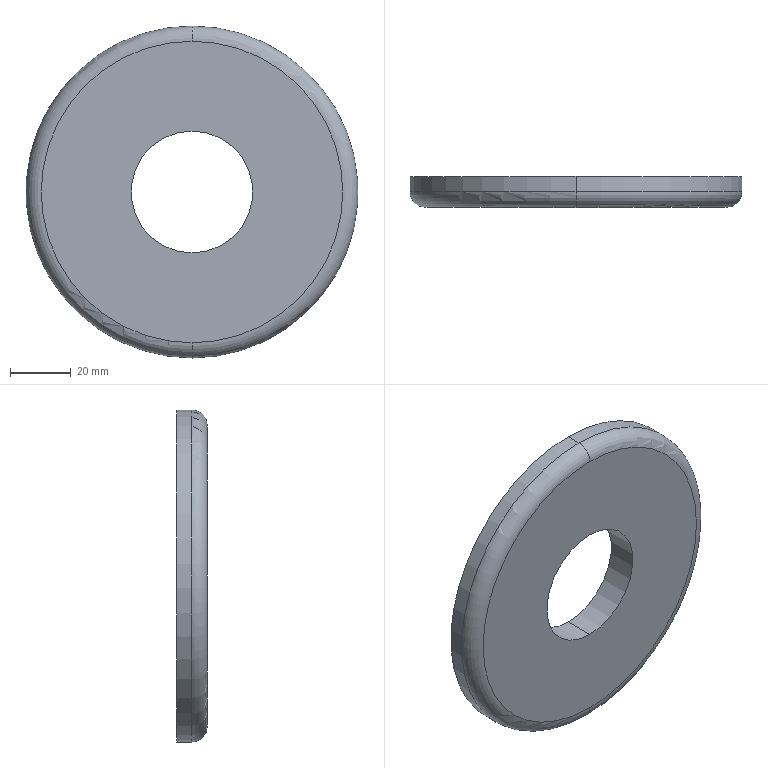Part | SolidWorks | features Revolution 1 | 1 solid | 8 faces | box 109 x 10 x 109 mm | volume 78947 mm3 | cylinder 4 | torus 2 | plane 2 | commonest cylinder face diameters 40 x2 109 x2
STEP:
#1=CARTESIAN_POINT('',(0.,-7.047,-20.));
#2=VERTEX_POINT('',#1);
#3=CARTESIAN_POINT('',(0.,-7.047,20.));
#4=VERTEX_POINT('',#3);
#5=CARTESIAN_POINT('',(0.,-7.047,0.));
#6=DIRECTION('',(0.,1.,0.));
#7=DIRECTION('',(0.,0.,1.));
#8=AXIS2_PLACEMENT_3D('',#5,#6,#7);
#9=CIRCLE('',#8,20.);
#10=EDGE_CURVE('',#2,#4,#9,.T.);
#11=ORIENTED_EDGE('',*,*,#10,.F.);
#12=CARTESIAN_POINT('',(0.,2.953,-20.));
#13=VERTEX_POINT('',#12);
#14=CARTESIAN_POINT('',(0.,51.821,-20.));
#15=DIRECTION('',(0.,1.,0.));
#16=VECTOR('',#15,1000.);
#17=LINE('',#14,#16);
#18=EDGE_CURVE('',#2,#13,#17,.T.);
#19=ORIENTED_EDGE('',*,*,#18,.T.);
#20=CARTESIAN_POINT('',(0.,2.953,20.));
#21=VERTEX_POINT('',#20);
#22=CARTESIAN_POINT('',(0.,2.953,0.));
#23=DIRECTION('',(0.,1.,0.));
#24=DIRECTION('',(0.,0.,1.));
#25=AXIS2_PLACEMENT_3D('',#22,#23,#24);
#26=CIRCLE('',#25,20.);
#27=EDGE_CURVE('',#13,#21,#26,.T.);
#28=ORIENTED_EDGE('',*,*,#27,.T.);
#29=CARTESIAN_POINT('',(0.,51.821,20.));
#30=DIRECTION('',(0.,1.,0.));
#31=VECTOR('',#30,1000.);
#32=LINE('',#29,#31);
#33=EDGE_CURVE('',#4,#21,#32,.T.);
#34=ORIENTED_EDGE('',*,*,#33,.F.);
#35=EDGE_LOOP('',(#11,#19,#28,#34));
#36=FACE_OUTER_BOUND('',#35,.T.);
#37=CARTESIAN_POINT('',(0.,51.821,0.));
#38=DIRECTION('',(0.,1.,0.));
#39=DIRECTION('',(0.,0.,1.));
#40=AXIS2_PLACEMENT_3D('',#37,#38,#39);
#41=CYLINDRICAL_SURFACE('',#40,20.);
#42=ADVANCED_FACE('',(#36),#41,.F.);
#43=CARTESIAN_POINT('',(0.,-2.047,54.5));
#44=VERTEX_POINT('',#43);
#45=CARTESIAN_POINT('',(0.,-2.047,-54.5));
#46=VERTEX_POINT('',#45);
#47=CARTESIAN_POINT('',(0.,-2.047,0.));
#48=DIRECTION('',(0.,1.,0.));
#49=DIRECTION('',(0.,0.,1.));
#50=AXIS2_PLACEMENT_3D('',#47,#48,#49);
#51=CIRCLE('',#50,54.5);
#52=EDGE_CURVE('',#44,#46,#51,.T.);
#53=ORIENTED_EDGE('',*,*,#52,.T.);
#54=CARTESIAN_POINT('',(0.,2.953,-54.5));
#55=VERTEX_POINT('',#54);
#56=CARTESIAN_POINT('',(0.,51.821,-54.5));
#57=DIRECTION('',(0.,1.,0.));
#58=VECTOR('',#57,1000.);
#59=LINE('',#56,#58);
#60=EDGE_CURVE('',#46,#55,#59,.T.);
#61=ORIENTED_EDGE('',*,*,#60,.T.);
#62=CARTESIAN_POINT('',(0.,2.953,54.5));
#63=VERTEX_POINT('',#62);
#64=CARTESIAN_POINT('',(0.,2.953,0.));
#65=DIRECTION('',(0.,1.,0.));
#66=DIRECTION('',(0.,0.,1.));
#67=AXIS2_PLACEMENT_3D('',#64,#65,#66);
#68=CIRCLE('',#67,54.5);
#69=EDGE_CURVE('',#63,#55,#68,.T.);
#70=ORIENTED_EDGE('',*,*,#69,.F.);
#71=CARTESIAN_POINT('',(0.,51.821,54.5));
#72=DIRECTION('',(0.,1.,0.));
#73=VECTOR('',#72,1000.);
#74=LINE('',#71,#73);
#75=EDGE_CURVE('',#44,#63,#74,.T.);
#76=ORIENTED_EDGE('',*,*,#75,.F.);
#77=EDGE_LOOP('',(#53,#61,#70,#76));
#78=FACE_OUTER_BOUND('',#77,.T.);
#79=CARTESIAN_POINT('',(0.,51.821,0.));
#80=DIRECTION('',(0.,1.,0.));
#81=DIRECTION('',(0.,0.,1.));
#82=AXIS2_PLACEMENT_3D('',#79,#80,#81);
#83=CYLINDRICAL_SURFACE('',#82,54.5);
#84=ADVANCED_FACE('',(#78),#83,.T.);
#85=CARTESIAN_POINT('',(0.,-7.047,49.5));
#86=VERTEX_POINT('',#85);
#87=CARTESIAN_POINT('',(0.,-7.047,-49.5));
#88=VERTEX_POINT('',#87);
#89=CARTESIAN_POINT('',(0.,-7.047,0.));
#90=DIRECTION('',(0.,1.,0.));
#91=DIRECTION('',(0.,0.,1.));
#92=AXIS2_PLACEMENT_3D('',#89,#90,#91);
#93=CIRCLE('',#92,49.5);
#94=EDGE_CURVE('',#86,#88,#93,.T.);
#95=ORIENTED_EDGE('',*,*,#94,.T.);
#96=CARTESIAN_POINT('',(0.,-2.047,-49.5));
#97=DIRECTION('',(1.,0.,0.));
#98=DIRECTION('',(0.,0.,-1.));
#99=AXIS2_PLACEMENT_3D('',#96,#97,#98);
#100=CIRCLE('',#99,5.);
#101=EDGE_CURVE('',#88,#46,#100,.T.);
#102=ORIENTED_EDGE('',*,*,#101,.T.);
#103=ORIENTED_EDGE('',*,*,#52,.F.);
#104=CARTESIAN_POINT('',(0.,-2.047,49.5));
#105=DIRECTION('',(-1.,0.,0.));
#106=DIRECTION('',(0.,0.,1.));
#107=AXIS2_PLACEMENT_3D('',#104,#105,#106);
#108=CIRCLE('',#107,5.);
#109=EDGE_CURVE('',#86,#44,#108,.T.);
#110=ORIENTED_EDGE('',*,*,#109,.F.);
#111=EDGE_LOOP('',(#95,#102,#103,#110));
#112=FACE_OUTER_BOUND('',#111,.T.);
#113=CARTESIAN_POINT('',(0.,-2.047,0.));
#114=DIRECTION('',(0.,1.,0.));
#115=DIRECTION('',(0.,0.,1.));
#116=AXIS2_PLACEMENT_3D('',#113,#114,#115);
#117=TOROIDAL_SURFACE('',#116,49.5,5.);
#118=ADVANCED_FACE('',(#112),#117,.T.);
#119=ORIENTED_EDGE('',*,*,#94,.F.);
#120=CARTESIAN_POINT('',(0.,-7.047,0.));
#121=DIRECTION('',(0.,1.,0.));
#122=DIRECTION('',(0.,0.,1.));
#123=AXIS2_PLACEMENT_3D('',#120,#121,#122);
#124=CIRCLE('',#123,49.5);
#125=EDGE_CURVE('',#88,#86,#124,.T.);
#126=ORIENTED_EDGE('',*,*,#125,.F.);
#127=EDGE_LOOP('',(#119,#126));
#128=FACE_OUTER_BOUND('',#127,.T.);
#129=CARTESIAN_POINT('',(0.,-7.047,0.));
#130=DIRECTION('',(0.,1.,0.));
#131=DIRECTION('',(0.,0.,1.));
#132=AXIS2_PLACEMENT_3D('',#129,#130,#131);
#133=CIRCLE('',#132,20.);
#134=EDGE_CURVE('',#4,#2,#133,.T.);
#135=ORIENTED_EDGE('',*,*,#134,.T.);
#136=ORIENTED_EDGE('',*,*,#10,.T.);
#137=EDGE_LOOP('',(#135,#136));
#138=FACE_BOUND('',#137,.T.);
#139=CARTESIAN_POINT('',(0.,-7.047,0.));
#140=DIRECTION('',(0.,1.,0.));
#141=DIRECTION('',(0.,0.,1.));
#142=AXIS2_PLACEMENT_3D('',#139,#140,#141);
#143=PLANE('',#142);
#144=ADVANCED_FACE('',(#128,#138),#143,.F.);
#145=ORIENTED_EDGE('',*,*,#101,.F.);
#146=ORIENTED_EDGE('',*,*,#125,.T.);
#147=ORIENTED_EDGE('',*,*,#109,.T.);
#148=CARTESIAN_POINT('',(0.,-2.047,0.));
#149=DIRECTION('',(0.,1.,0.));
#150=DIRECTION('',(0.,0.,1.));
#151=AXIS2_PLACEMENT_3D('',#148,#149,#150);
#152=CIRCLE('',#151,54.5);
#153=EDGE_CURVE('',#46,#44,#152,.T.);
#154=ORIENTED_EDGE('',*,*,#153,.F.);
#155=EDGE_LOOP('',(#145,#146,#147,#154));
#156=FACE_OUTER_BOUND('',#155,.T.);
#157=CARTESIAN_POINT('',(0.,-2.047,0.));
#158=DIRECTION('',(0.,1.,0.));
#159=DIRECTION('',(0.,0.,1.));
#160=AXIS2_PLACEMENT_3D('',#157,#158,#159);
#161=TOROIDAL_SURFACE('',#160,49.5,5.);
#162=ADVANCED_FACE('',(#156),#161,.T.);
#163=ORIENTED_EDGE('',*,*,#60,.F.);
#164=ORIENTED_EDGE('',*,*,#153,.T.);
#165=ORIENTED_EDGE('',*,*,#75,.T.);
#166=CARTESIAN_POINT('',(0.,2.953,0.));
#167=DIRECTION('',(0.,1.,0.));
#168=DIRECTION('',(0.,0.,1.));
#169=AXIS2_PLACEMENT_3D('',#166,#167,#168);
#170=CIRCLE('',#169,54.5);
#171=EDGE_CURVE('',#55,#63,#170,.T.);
#172=ORIENTED_EDGE('',*,*,#171,.F.);
#173=EDGE_LOOP('',(#163,#164,#165,#172));
#174=FACE_OUTER_BOUND('',#173,.T.);
#175=CARTESIAN_POINT('',(0.,51.821,0.));
#176=DIRECTION('',(0.,1.,0.));
#177=DIRECTION('',(0.,0.,1.));
#178=AXIS2_PLACEMENT_3D('',#175,#176,#177);
#179=CYLINDRICAL_SURFACE('',#178,54.5);
#180=ADVANCED_FACE('',(#174),#179,.T.);
#181=CARTESIAN_POINT('',(0.,2.953,0.));
#182=DIRECTION('',(0.,1.,0.));
#183=DIRECTION('',(0.,0.,1.));
#184=AXIS2_PLACEMENT_3D('',#181,#182,#183);
#185=CIRCLE('',#184,20.);
#186=EDGE_CURVE('',#21,#13,#185,.T.);
#187=ORIENTED_EDGE('',*,*,#186,.F.);
#188=ORIENTED_EDGE('',*,*,#27,.F.);
#189=EDGE_LOOP('',(#187,#188));
#190=FACE_BOUND('',#189,.T.);
#191=ORIENTED_EDGE('',*,*,#69,.T.);
#192=ORIENTED_EDGE('',*,*,#171,.T.);
#193=EDGE_LOOP('',(#191,#192));
#194=FACE_OUTER_BOUND('',#193,.T.);
#195=CARTESIAN_POINT('',(0.,2.953,0.));
#196=DIRECTION('',(0.,-1.,0.));
#197=DIRECTION('',(0.,0.,-1.));
#198=AXIS2_PLACEMENT_3D('',#195,#196,#197);
#199=PLANE('',#198);
#200=ADVANCED_FACE('',(#190,#194),#199,.F.);
#201=ORIENTED_EDGE('',*,*,#18,.F.);
#202=ORIENTED_EDGE('',*,*,#134,.F.);
#203=ORIENTED_EDGE('',*,*,#33,.T.);
#204=ORIENTED_EDGE('',*,*,#186,.T.);
#205=EDGE_LOOP('',(#201,#202,#203,#204));
#206=FACE_OUTER_BOUND('',#205,.T.);
#207=CARTESIAN_POINT('',(0.,51.821,0.));
#208=DIRECTION('',(0.,1.,0.));
#209=DIRECTION('',(0.,0.,1.));
#210=AXIS2_PLACEMENT_3D('',#207,#208,#209);
#211=CYLINDRICAL_SURFACE('',#210,20.);
#212=ADVANCED_FACE('',(#206),#211,.F.);
#213=CLOSED_SHELL('',(#42,#84,#118,#144,#162,#180,#200,#212));
#214=MANIFOLD_SOLID_BREP('',#213);
#215=CARTESIAN_POINT('',(0.,0.,0.));
#216=DIRECTION('',(0.,0.,1.));
#217=DIRECTION('',(1.,0.,0.));
#218=AXIS2_PLACEMENT_3D('',#215,#216,#217);
#219=(LENGTH_UNIT()NAMED_UNIT(*)SI_UNIT(.MILLI.,.METRE.));
#220=UNCERTAINTY_MEASURE_WITH_UNIT(LENGTH_MEASURE(0.00001),#219,'','');
#221=(NAMED_UNIT(*)PLANE_ANGLE_UNIT()SI_UNIT($,.RADIAN.));
#222=(NAMED_UNIT(*)SI_UNIT($,.STERADIAN.)SOLID_ANGLE_UNIT());
#223=(GEOMETRIC_REPRESENTATION_CONTEXT(3)GLOBAL_UNCERTAINTY_ASSIGNED_CONTEXT((#220))GLOBAL_UNIT_ASSIGNED_CONTEXT((#219,#221,#222))REPRESENTATION_CONTEXT('',''));
#224=ADVANCED_BREP_SHAPE_REPRESENTATION('',(#214,#218),#223);